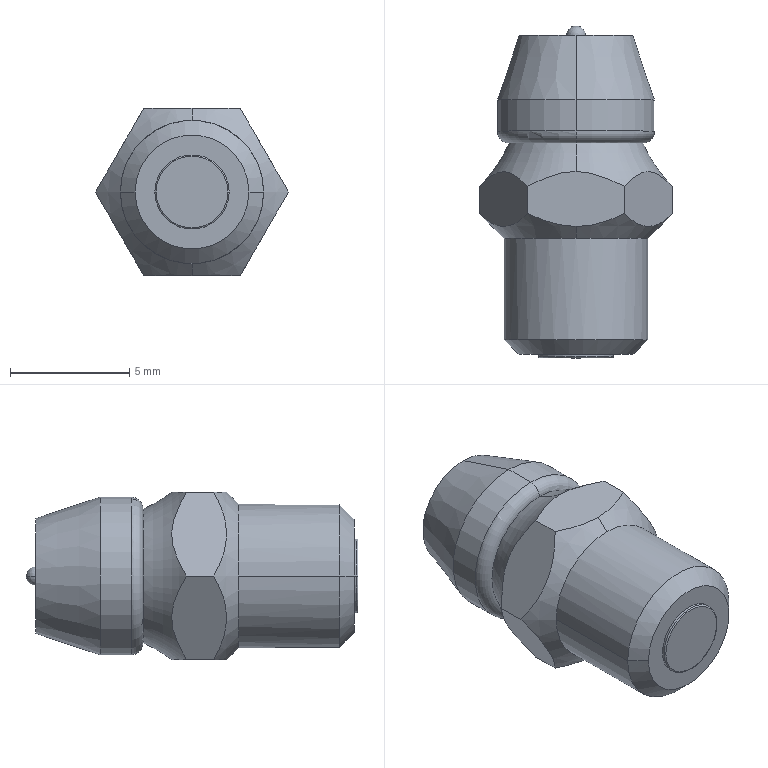Part | STEP file | GPAS6A-4 | 1 solid | 29 faces | box 8.083 x 13.9 x 7 mm | volume 414.719 mm3 | plane 9 | cylinder 6 | cone 6 | torus 6 | sphere 2 | commonest cylinder face diameters 3.113 x2 6 x2 6.6 x2
STEP:
#1=CARTESIAN_POINT('',(-3.,-5.986,0.));
#2=VERTEX_POINT('',#1);
#3=CARTESIAN_POINT('',(3.,-5.986,0.));
#4=VERTEX_POINT('',#3);
#5=CARTESIAN_POINT('',(0.,-5.986,0.));
#6=DIRECTION('',(0.,1.,0.));
#7=DIRECTION('',(-1.,0.,0.));
#8=AXIS2_PLACEMENT_3D('',#5,#6,#7);
#9=CIRCLE('',#8,3.);
#10=EDGE_CURVE('',#2,#4,#9,.T.);
#11=ORIENTED_EDGE('',*,*,#10,.T.);
#12=CARTESIAN_POINT('',(3.,-1.75,0.));
#13=VERTEX_POINT('',#12);
#14=CARTESIAN_POINT('',(3.,-1.75,0.));
#15=DIRECTION('',(0.,1.,0.));
#16=VECTOR('',#15,1000.);
#17=LINE('',#14,#16);
#18=EDGE_CURVE('',#4,#13,#17,.T.);
#19=ORIENTED_EDGE('',*,*,#18,.T.);
#20=CARTESIAN_POINT('',(0.,-1.75,3.));
#21=VERTEX_POINT('',#20);
#22=CARTESIAN_POINT('',(0.,-1.75,0.));
#23=DIRECTION('',(0.,1.,0.));
#24=DIRECTION('',(-1.,0.,0.));
#25=AXIS2_PLACEMENT_3D('',#22,#23,#24);
#26=CIRCLE('',#25,3.);
#27=EDGE_CURVE('',#21,#13,#26,.T.);
#28=ORIENTED_EDGE('',*,*,#27,.F.);
#29=CARTESIAN_POINT('',(-3.,-1.75,0.));
#30=VERTEX_POINT('',#29);
#31=CARTESIAN_POINT('',(0.,-1.75,0.));
#32=DIRECTION('',(0.,1.,0.));
#33=DIRECTION('',(-1.,0.,0.));
#34=AXIS2_PLACEMENT_3D('',#31,#32,#33);
#35=CIRCLE('',#34,3.);
#36=EDGE_CURVE('',#30,#21,#35,.T.);
#37=ORIENTED_EDGE('',*,*,#36,.F.);
#38=CARTESIAN_POINT('',(-3.,-1.75,0.));
#39=DIRECTION('',(0.,1.,0.));
#40=VECTOR('',#39,1000.);
#41=LINE('',#38,#40);
#42=EDGE_CURVE('',#2,#30,#41,.T.);
#43=ORIENTED_EDGE('',*,*,#42,.F.);
#44=EDGE_LOOP('',(#11,#19,#28,#37,#43));
#45=FACE_OUTER_BOUND('',#44,.T.);
#46=CARTESIAN_POINT('',(0.,-1.75,0.));
#47=DIRECTION('',(0.,1.,0.));
#48=DIRECTION('',(-1.,0.,0.));
#49=AXIS2_PLACEMENT_3D('',#46,#47,#48);
#50=CYLINDRICAL_SURFACE('',#49,3.);
#51=ADVANCED_FACE('',(#45),#50,.T.);
#52=CARTESIAN_POINT('',(-2.387,-6.6,0.));
#53=VERTEX_POINT('',#52);
#54=CARTESIAN_POINT('',(2.387,-6.6,0.));
#55=VERTEX_POINT('',#54);
#56=CARTESIAN_POINT('',(0.,-6.6,0.));
#57=DIRECTION('',(0.,1.,0.));
#58=DIRECTION('',(-1.,0.,0.));
#59=AXIS2_PLACEMENT_3D('',#56,#57,#58);
#60=CIRCLE('',#59,2.387);
#61=EDGE_CURVE('',#53,#55,#60,.T.);
#62=ORIENTED_EDGE('',*,*,#61,.T.);
#63=CARTESIAN_POINT('',(2.387,-6.6,0.));
#64=DIRECTION('',(0.7071,0.7071,0.));
#65=VECTOR('',#64,1000.);
#66=LINE('',#63,#65);
#67=EDGE_CURVE('',#55,#4,#66,.T.);
#68=ORIENTED_EDGE('',*,*,#67,.T.);
#69=ORIENTED_EDGE('',*,*,#10,.F.);
#70=CARTESIAN_POINT('',(-2.387,-6.6,0.));
#71=DIRECTION('',(-0.7071,0.7071,0.));
#72=VECTOR('',#71,1000.);
#73=LINE('',#70,#72);
#74=EDGE_CURVE('',#53,#2,#73,.T.);
#75=ORIENTED_EDGE('',*,*,#74,.F.);
#76=EDGE_LOOP('',(#62,#68,#69,#75));
#77=FACE_OUTER_BOUND('',#76,.T.);
#78=CARTESIAN_POINT('',(0.,-6.6,0.));
#79=DIRECTION('',(0.,1.,0.));
#80=DIRECTION('',(-1.,0.,0.));
#81=AXIS2_PLACEMENT_3D('',#78,#79,#80);
#82=CONICAL_SURFACE('',#81,2.387,0.7854);
#83=ADVANCED_FACE('',(#77),#82,.T.);
#84=CARTESIAN_POINT('',(-1.556,-6.698,0.));
#85=VERTEX_POINT('',#84);
#86=CARTESIAN_POINT('',(1.556,-6.698,0.));
#87=VERTEX_POINT('',#86);
#88=CARTESIAN_POINT('',(0.,-6.698,0.));
#89=DIRECTION('',(0.,1.,0.));
#90=DIRECTION('',(-1.,0.,0.));
#91=AXIS2_PLACEMENT_3D('',#88,#89,#90);
#92=CIRCLE('',#91,1.556);
#93=EDGE_CURVE('',#85,#87,#92,.T.);
#94=ORIENTED_EDGE('',*,*,#93,.T.);
#95=CARTESIAN_POINT('',(1.556,-6.6,0.));
#96=VERTEX_POINT('',#95);
#97=CARTESIAN_POINT('',(1.556,-1.75,0.));
#98=DIRECTION('',(0.,1.,0.));
#99=VECTOR('',#98,1000.);
#100=LINE('',#97,#99);
#101=EDGE_CURVE('',#87,#96,#100,.T.);
#102=ORIENTED_EDGE('',*,*,#101,.T.);
#103=CARTESIAN_POINT('',(-1.556,-6.6,0.));
#104=VERTEX_POINT('',#103);
#105=CARTESIAN_POINT('',(0.,-6.6,0.));
#106=DIRECTION('',(0.,1.,0.));
#107=DIRECTION('',(-1.,0.,0.));
#108=AXIS2_PLACEMENT_3D('',#105,#106,#107);
#109=CIRCLE('',#108,1.556);
#110=EDGE_CURVE('',#104,#96,#109,.T.);
#111=ORIENTED_EDGE('',*,*,#110,.F.);
#112=CARTESIAN_POINT('',(-1.556,-1.75,0.));
#113=DIRECTION('',(0.,1.,0.));
#114=VECTOR('',#113,1000.);
#115=LINE('',#112,#114);
#116=EDGE_CURVE('',#85,#104,#115,.T.);
#117=ORIENTED_EDGE('',*,*,#116,.F.);
#118=EDGE_LOOP('',(#94,#102,#111,#117));
#119=FACE_OUTER_BOUND('',#118,.T.);
#120=CARTESIAN_POINT('',(0.,-1.75,0.));
#121=DIRECTION('',(0.,1.,0.));
#122=DIRECTION('',(-1.,0.,0.));
#123=AXIS2_PLACEMENT_3D('',#120,#121,#122);
#124=CYLINDRICAL_SURFACE('',#123,1.556);
#125=ADVANCED_FACE('',(#119),#124,.T.);
#126=CARTESIAN_POINT('',(-1.505,-6.75,0.));
#127=VERTEX_POINT('',#126);
#128=CARTESIAN_POINT('',(1.505,-6.75,0.));
#129=VERTEX_POINT('',#128);
#130=CARTESIAN_POINT('',(0.,-6.75,0.));
#131=DIRECTION('',(0.,1.,0.));
#132=DIRECTION('',(-1.,0.,0.));
#133=AXIS2_PLACEMENT_3D('',#130,#131,#132);
#134=CIRCLE('',#133,1.505);
#135=EDGE_CURVE('',#127,#129,#134,.T.);
#136=ORIENTED_EDGE('',*,*,#135,.T.);
#137=CARTESIAN_POINT('',(1.505,-6.698,0.));
#138=DIRECTION('',(0.,0.,1.));
#139=DIRECTION('',(1.,0.,0.));
#140=AXIS2_PLACEMENT_3D('',#137,#138,#139);
#141=CIRCLE('',#140,0.05188);
#142=EDGE_CURVE('',#129,#87,#141,.T.);
#143=ORIENTED_EDGE('',*,*,#142,.T.);
#144=ORIENTED_EDGE('',*,*,#93,.F.);
#145=CARTESIAN_POINT('',(-1.505,-6.698,0.));
#146=DIRECTION('',(0.,0.,-1.));
#147=DIRECTION('',(-1.,0.,0.));
#148=AXIS2_PLACEMENT_3D('',#145,#146,#147);
#149=CIRCLE('',#148,0.05188);
#150=EDGE_CURVE('',#127,#85,#149,.T.);
#151=ORIENTED_EDGE('',*,*,#150,.F.);
#152=EDGE_LOOP('',(#136,#143,#144,#151));
#153=FACE_OUTER_BOUND('',#152,.T.);
#154=CARTESIAN_POINT('',(0.,-6.698,0.));
#155=DIRECTION('',(0.,1.,0.));
#156=DIRECTION('',(-1.,0.,0.));
#157=AXIS2_PLACEMENT_3D('',#154,#155,#156);
#158=TOROIDAL_SURFACE('',#157,1.505,0.05188);
#159=ADVANCED_FACE('',(#153),#158,.T.);
#160=CARTESIAN_POINT('',(0.4,6.75,0.));
#161=VERTEX_POINT('',#160);
#162=CARTESIAN_POINT('',(-0.4,6.75,0.));
#163=VERTEX_POINT('',#162);
#164=CARTESIAN_POINT('',(0.,6.75,0.));
#165=DIRECTION('',(0.,1.,0.));
#166=DIRECTION('',(0.,0.,1.));
#167=AXIS2_PLACEMENT_3D('',#164,#165,#166);
#168=CIRCLE('',#167,0.4);
#169=EDGE_CURVE('',#161,#163,#168,.T.);
#170=ORIENTED_EDGE('',*,*,#169,.T.);
#171=CARTESIAN_POINT('',(0.,7.15,0.));
#172=VERTEX_POINT('',#171);
#173=CARTESIAN_POINT('',(0.,6.75,0.));
#174=DIRECTION('',(0.,0.,-1.));
#175=DIRECTION('',(-1.,0.,0.));
#176=AXIS2_PLACEMENT_3D('',#173,#174,#175);
#177=CIRCLE('',#176,0.4);
#178=EDGE_CURVE('',#163,#172,#177,.T.);
#179=ORIENTED_EDGE('',*,*,#178,.T.);
#180=CARTESIAN_POINT('',(0.,6.75,0.));
#181=DIRECTION('',(0.,0.,1.));
#182=DIRECTION('',(1.,0.,0.));
#183=AXIS2_PLACEMENT_3D('',#180,#181,#182);
#184=CIRCLE('',#183,0.4);
#185=EDGE_CURVE('',#161,#172,#184,.T.);
#186=ORIENTED_EDGE('',*,*,#185,.F.);
#187=EDGE_LOOP('',(#170,#179,#186));
#188=FACE_OUTER_BOUND('',#187,.T.);
#189=CARTESIAN_POINT('',(0.,6.75,0.));
#190=DIRECTION('',(0.,0.,-1.));
#191=DIRECTION('',(1.,0.,0.));
#192=AXIS2_PLACEMENT_3D('',#189,#190,#191);
#193=SPHERICAL_SURFACE('',#192,0.4);
#194=ADVANCED_FACE('',(#188),#193,.T.);
#195=CARTESIAN_POINT('',(0.,6.75,2.4));
#196=VERTEX_POINT('',#195);
#197=CARTESIAN_POINT('',(0.,6.75,-2.4));
#198=VERTEX_POINT('',#197);
#199=CARTESIAN_POINT('',(0.,6.75,0.));
#200=DIRECTION('',(0.,1.,0.));
#201=DIRECTION('',(0.,0.,1.));
#202=AXIS2_PLACEMENT_3D('',#199,#200,#201);
#203=CIRCLE('',#202,2.4);
#204=EDGE_CURVE('',#196,#198,#203,.T.);
#205=ORIENTED_EDGE('',*,*,#204,.F.);
#206=CARTESIAN_POINT('',(0.,4.05,3.3));
#207=VERTEX_POINT('',#206);
#208=CARTESIAN_POINT('',(0.,4.05,3.3));
#209=DIRECTION('',(0.,-0.9487,0.3162));
#210=VECTOR('',#209,1000.);
#211=LINE('',#208,#210);
#212=EDGE_CURVE('',#196,#207,#211,.T.);
#213=ORIENTED_EDGE('',*,*,#212,.T.);
#214=CARTESIAN_POINT('',(0.,4.05,-3.3));
#215=VERTEX_POINT('',#214);
#216=CARTESIAN_POINT('',(0.,4.05,0.));
#217=DIRECTION('',(0.,1.,0.));
#218=DIRECTION('',(0.,0.,1.));
#219=AXIS2_PLACEMENT_3D('',#216,#217,#218);
#220=CIRCLE('',#219,3.3);
#221=EDGE_CURVE('',#207,#215,#220,.T.);
#222=ORIENTED_EDGE('',*,*,#221,.T.);
#223=CARTESIAN_POINT('',(0.,4.05,-3.3));
#224=DIRECTION('',(0.,-0.9487,-0.3162));
#225=VECTOR('',#224,1000.);
#226=LINE('',#223,#225);
#227=EDGE_CURVE('',#198,#215,#226,.T.);
#228=ORIENTED_EDGE('',*,*,#227,.F.);
#229=EDGE_LOOP('',(#205,#213,#222,#228));
#230=FACE_OUTER_BOUND('',#229,.T.);
#231=CARTESIAN_POINT('',(0.,4.05,0.));
#232=DIRECTION('',(0.,-1.,0.));
#233=DIRECTION('',(0.,0.,-1.));
#234=AXIS2_PLACEMENT_3D('',#231,#232,#233);
#235=CONICAL_SURFACE('',#234,3.3,0.3218);
#236=ADVANCED_FACE('',(#230),#235,.T.);
#237=CARTESIAN_POINT('',(0.,2.75,3.3));
#238=VERTEX_POINT('',#237);
#239=CARTESIAN_POINT('',(0.,2.75,-3.3));
#240=VERTEX_POINT('',#239);
#241=CARTESIAN_POINT('',(0.,2.75,0.));
#242=DIRECTION('',(0.,1.,0.));
#243=DIRECTION('',(0.,0.,1.));
#244=AXIS2_PLACEMENT_3D('',#241,#242,#243);
#245=CIRCLE('',#244,3.3);
#246=EDGE_CURVE('',#238,#240,#245,.T.);
#247=ORIENTED_EDGE('',*,*,#246,.T.);
#248=CARTESIAN_POINT('',(0.,6.75,-3.3));
#249=DIRECTION('',(0.,1.,0.));
#250=VECTOR('',#249,1000.);
#251=LINE('',#248,#250);
#252=EDGE_CURVE('',#240,#215,#251,.T.);
#253=ORIENTED_EDGE('',*,*,#252,.T.);
#254=ORIENTED_EDGE('',*,*,#221,.F.);
#255=CARTESIAN_POINT('',(0.,6.75,3.3));
#256=DIRECTION('',(0.,1.,0.));
#257=VECTOR('',#256,1000.);
#258=LINE('',#255,#257);
#259=EDGE_CURVE('',#238,#207,#258,.T.);
#260=ORIENTED_EDGE('',*,*,#259,.F.);
#261=EDGE_LOOP('',(#247,#253,#254,#260));
#262=FACE_OUTER_BOUND('',#261,.T.);
#263=CARTESIAN_POINT('',(0.,6.75,0.));
#264=DIRECTION('',(0.,1.,0.));
#265=DIRECTION('',(0.,0.,1.));
#266=AXIS2_PLACEMENT_3D('',#263,#264,#265);
#267=CYLINDRICAL_SURFACE('',#266,3.3);
#268=ADVANCED_FACE('',(#262),#267,.T.);
#269=CARTESIAN_POINT('',(0.,2.25,2.8));
#270=VERTEX_POINT('',#269);
#271=CARTESIAN_POINT('',(0.,2.25,-2.8));
#272=VERTEX_POINT('',#271);
#273=CARTESIAN_POINT('',(0.,2.25,0.));
#274=DIRECTION('',(0.,1.,0.));
#275=DIRECTION('',(0.,0.,1.));
#276=AXIS2_PLACEMENT_3D('',#273,#274,#275);
#277=CIRCLE('',#276,2.8);
#278=EDGE_CURVE('',#270,#272,#277,.T.);
#279=ORIENTED_EDGE('',*,*,#278,.T.);
#280=CARTESIAN_POINT('',(0.,2.75,-2.8));
#281=DIRECTION('',(1.,0.,0.));
#282=DIRECTION('',(0.,0.,-1.));
#283=AXIS2_PLACEMENT_3D('',#280,#281,#282);
#284=CIRCLE('',#283,0.5);
#285=EDGE_CURVE('',#272,#240,#284,.T.);
#286=ORIENTED_EDGE('',*,*,#285,.T.);
#287=ORIENTED_EDGE('',*,*,#246,.F.);
#288=CARTESIAN_POINT('',(0.,2.75,2.8));
#289=DIRECTION('',(-1.,0.,0.));
#290=DIRECTION('',(0.,0.,1.));
#291=AXIS2_PLACEMENT_3D('',#288,#289,#290);
#292=CIRCLE('',#291,0.5);
#293=EDGE_CURVE('',#270,#238,#292,.T.);
#294=ORIENTED_EDGE('',*,*,#293,.F.);
#295=EDGE_LOOP('',(#279,#286,#287,#294));
#296=FACE_OUTER_BOUND('',#295,.T.);
#297=CARTESIAN_POINT('',(0.,2.75,0.));
#298=DIRECTION('',(0.,1.,0.));
#299=DIRECTION('',(0.,0.,1.));
#300=AXIS2_PLACEMENT_3D('',#297,#298,#299);
#301=TOROIDAL_SURFACE('',#300,2.8,0.5);
#302=ADVANCED_FACE('',(#296),#301,.T.);
#303=CARTESIAN_POINT('',(0.,2.25,0.));
#304=DIRECTION('',(0.,1.,0.));
#305=DIRECTION('',(0.,0.,1.));
#306=AXIS2_PLACEMENT_3D('',#303,#304,#305);
#307=CIRCLE('',#306,2.8);
#308=EDGE_CURVE('',#272,#270,#307,.T.);
#309=ORIENTED_EDGE('',*,*,#308,.F.);
#310=CARTESIAN_POINT('',(0.,1.053,-3.5));
#311=VERTEX_POINT('',#310);
#312=CARTESIAN_POINT('',(0.,4.661,-8.294));
#313=DIRECTION('',(1.,0.,0.));
#314=DIRECTION('',(0.,0.,-1.));
#315=AXIS2_PLACEMENT_3D('',#312,#313,#314);
#316=CIRCLE('',#315,6.);
#317=EDGE_CURVE('',#272,#311,#316,.T.);
#318=ORIENTED_EDGE('',*,*,#317,.T.);
#319=CARTESIAN_POINT('',(-2.021,0.4286,-3.5));
#320=VERTEX_POINT('',#319);
#321=CARTESIAN_POINT('',(0.,1.053,-3.5));
#322=CARTESIAN_POINT('',(-0.1777,1.053,-3.5));
#323=CARTESIAN_POINT('',(-0.3562,1.035,-3.5));
#324=CARTESIAN_POINT('',(-0.7092,0.9659,-3.5));
#325=CARTESIAN_POINT('',(-0.88,0.9167,-3.5));
#326=CARTESIAN_POINT('',(-1.382,0.7411,-3.5));
#327=CARTESIAN_POINT('',(-1.703,0.5884,-3.5));
#328=CARTESIAN_POINT('',(-2.021,0.4286,-3.5));
#329=B_SPLINE_CURVE_WITH_KNOTS('',3,(#321,#322,#323,#324,#325,#326,#327,#328),.UNSPECIFIED.,.F.,.F.,(4,2,2,4),(0.00693,0.007463,0.007996,0.009062),.UNSPECIFIED.);
#330=EDGE_CURVE('',#311,#320,#329,.T.);
#331=ORIENTED_EDGE('',*,*,#330,.T.);
#332=CARTESIAN_POINT('',(-4.041,0.4286,0.));
#333=VERTEX_POINT('',#332);
#334=CARTESIAN_POINT('',(-2.021,0.4286,-3.5));
#335=CARTESIAN_POINT('',(-2.18,0.5886,-3.224));
#336=CARTESIAN_POINT('',(-2.341,0.7417,-2.946));
#337=CARTESIAN_POINT('',(-2.593,0.9177,-2.509));
#338=CARTESIAN_POINT('',(-2.679,0.9672,-2.359));
#339=CARTESIAN_POINT('',(-2.854,1.035,-2.057));
#340=CARTESIAN_POINT('',(-2.942,1.053,-1.904));
#341=CARTESIAN_POINT('',(-3.12,1.053,-1.597));
#342=CARTESIAN_POINT('',(-3.21,1.035,-1.441));
#343=CARTESIAN_POINT('',(-3.384,0.9667,-1.139));
#344=CARTESIAN_POINT('',(-3.469,0.9179,-0.9914));
#345=CARTESIAN_POINT('',(-3.72,0.7428,-0.5566));
#346=CARTESIAN_POINT('',(-3.882,0.5887,-0.2761));
#347=CARTESIAN_POINT('',(-4.041,0.4286,0.));
#348=B_SPLINE_CURVE_WITH_KNOTS('',3,(#334,#335,#336,#337,#338,#339,#340,#341,#342,#343,#344,#345,#346,#347),.UNSPECIFIED.,.F.,.F.,(4,2,2,2,2,2,4),(0.000000258,0.001066,0.001599,0.002132,0.002666,0.003199,0.004265),.UNSPECIFIED.);
#349=EDGE_CURVE('',#320,#333,#348,.T.);
#350=ORIENTED_EDGE('',*,*,#349,.T.);
#351=CARTESIAN_POINT('',(-2.021,0.4286,3.5));
#352=VERTEX_POINT('',#351);
#353=CARTESIAN_POINT('',(-4.041,0.4286,0.));
#354=CARTESIAN_POINT('',(-3.882,0.5886,0.2759));
#355=CARTESIAN_POINT('',(-3.721,0.7417,0.5542));
#356=CARTESIAN_POINT('',(-3.47,0.9177,0.9906));
#357=CARTESIAN_POINT('',(-3.383,0.9672,1.141));
#358=CARTESIAN_POINT('',(-3.208,1.035,1.443));
#359=CARTESIAN_POINT('',(-3.12,1.053,1.596));
#360=CARTESIAN_POINT('',(-2.943,1.053,1.903));
#361=CARTESIAN_POINT('',(-2.853,1.035,2.059));
#362=CARTESIAN_POINT('',(-2.678,0.9667,2.361));
#363=CARTESIAN_POINT('',(-2.593,0.9179,2.509));
#364=CARTESIAN_POINT('',(-2.342,0.7428,2.943));
#365=CARTESIAN_POINT('',(-2.18,0.5887,3.224));
#366=CARTESIAN_POINT('',(-2.021,0.4286,3.5));
#367=B_SPLINE_CURVE_WITH_KNOTS('',3,(#353,#354,#355,#356,#357,#358,#359,#360,#361,#362,#363,#364,#365,#366),.UNSPECIFIED.,.F.,.F.,(4,2,2,2,2,2,4),(0.000000258,0.001066,0.001599,0.002132,0.002666,0.003199,0.004265),.UNSPECIFIED.);
#368=EDGE_CURVE('',#333,#352,#367,.T.);
#369=ORIENTED_EDGE('',*,*,#368,.T.);
#370=CARTESIAN_POINT('',(0.,1.053,3.5));
#371=VERTEX_POINT('',#370);
#372=CARTESIAN_POINT('',(-2.021,0.4286,3.5));
#373=CARTESIAN_POINT('',(-1.702,0.5886,3.5));
#374=CARTESIAN_POINT('',(-1.379,0.7424,3.5));
#375=CARTESIAN_POINT('',(-0.8765,0.9178,3.5));
#376=CARTESIAN_POINT('',(-0.7058,0.9668,3.5));
#377=CARTESIAN_POINT('',(-0.3544,1.035,3.5));
#378=CARTESIAN_POINT('',(-0.1767,1.053,3.5));
#379=CARTESIAN_POINT('',(0.,1.053,3.5));
#380=B_SPLINE_CURVE_WITH_KNOTS('',3,(#372,#373,#374,#375,#376,#377,#378,#379),.UNSPECIFIED.,.F.,.F.,(4,2,2,4),(0.004809,0.00587,0.0064,0.00693),.UNSPECIFIED.);
#381=EDGE_CURVE('',#352,#371,#380,.T.);
#382=ORIENTED_EDGE('',*,*,#381,.T.);
#383=CARTESIAN_POINT('',(0.,4.661,8.294));
#384=DIRECTION('',(-1.,0.,0.));
#385=DIRECTION('',(0.,0.,1.));
#386=AXIS2_PLACEMENT_3D('',#383,#384,#385);
#387=CIRCLE('',#386,6.);
#388=EDGE_CURVE('',#270,#371,#387,.T.);
#389=ORIENTED_EDGE('',*,*,#388,.F.);
#390=EDGE_LOOP('',(#309,#318,#331,#350,#369,#382,#389));
#391=FACE_OUTER_BOUND('',#390,.T.);
#392=CARTESIAN_POINT('',(0.,4.661,0.));
#393=DIRECTION('',(0.,1.,0.));
#394=DIRECTION('',(0.,0.,1.));
#395=AXIS2_PLACEMENT_3D('',#392,#393,#394);
#396=TOROIDAL_SURFACE('',#395,8.294,6.);
#397=ADVANCED_FACE('',(#391),#396,.F.);
#398=ORIENTED_EDGE('',*,*,#27,.T.);
#399=CARTESIAN_POINT('',(0.,-1.75,-3.));
#400=VERTEX_POINT('',#399);
#401=CARTESIAN_POINT('',(0.,-1.75,0.));
#402=DIRECTION('',(0.,1.,0.));
#403=DIRECTION('',(-1.,0.,0.));
#404=AXIS2_PLACEMENT_3D('',#401,#402,#403);
#405=CIRCLE('',#404,3.);
#406=EDGE_CURVE('',#13,#400,#405,.T.);
#407=ORIENTED_EDGE('',*,*,#406,.T.);
#408=CARTESIAN_POINT('',(0.,-1.25,-3.5));
#409=VERTEX_POINT('',#408);
#410=CARTESIAN_POINT('',(0.,-1.8,-2.95));
#411=DIRECTION('',(0.,0.7071,-0.7071));
#412=VECTOR('',#411,1000.);
#413=LINE('',#410,#412);
#414=EDGE_CURVE('',#400,#409,#413,.T.);
#415=ORIENTED_EDGE('',*,*,#414,.T.);
#416=CARTESIAN_POINT('',(2.021,-0.7085,-3.5));
#417=VERTEX_POINT('',#416);
#418=CARTESIAN_POINT('',(0.,-1.25,-3.5));
#419=CARTESIAN_POINT('',(0.1774,-1.25,-3.5));
#420=CARTESIAN_POINT('',(0.3548,-1.236,-3.5));
#421=CARTESIAN_POINT('',(0.7015,-1.185,-3.5));
#422=CARTESIAN_POINT('',(0.8722,-1.147,-3.5));
#423=CARTESIAN_POINT('',(1.377,-1.003,-3.5));
#424=CARTESIAN_POINT('',(1.707,-0.8653,-3.5));
#425=CARTESIAN_POINT('',(2.021,-0.7085,-3.5));
#426=B_SPLINE_CURVE_WITH_KNOTS('',3,(#418,#419,#420,#421,#422,#423,#424,#425),.UNSPECIFIED.,.F.,.F.,(4,2,2,4),(0.007385,0.007911,0.008437,0.009489),.UNSPECIFIED.);
#427=EDGE_CURVE('',#409,#417,#426,.T.);
#428=ORIENTED_EDGE('',*,*,#427,.T.);
#429=CARTESIAN_POINT('',(4.041,-0.7085,0.));
#430=VERTEX_POINT('',#429);
#431=CARTESIAN_POINT('',(2.021,-0.7085,-3.5));
#432=CARTESIAN_POINT('',(2.179,-0.8664,-3.227));
#433=CARTESIAN_POINT('',(2.34,-1.001,-2.947));
#434=CARTESIAN_POINT('',(2.591,-1.145,-2.512));
#435=CARTESIAN_POINT('',(2.676,-1.183,-2.365));
#436=CARTESIAN_POINT('',(2.85,-1.235,-2.064));
#437=CARTESIAN_POINT('',(2.939,-1.25,-1.909));
#438=CARTESIAN_POINT('',(3.204,-1.251,-1.451));
#439=CARTESIAN_POINT('',(3.377,-1.197,-1.151));
#440=CARTESIAN_POINT('',(3.719,-1.004,-0.5583));
#441=CARTESIAN_POINT('',(3.883,-0.8674,-0.2751));
#442=CARTESIAN_POINT('',(4.041,-0.7085,0.));
#443=B_SPLINE_CURVE_WITH_KNOTS('',3,(#431,#432,#433,#434,#435,#436,#437,#438,#439,#440,#441,#442),.UNSPECIFIED.,.F.,.F.,(4,2,2,2,2,4),(0.000000254,0.001044,0.001566,0.002088,0.003131,0.004175),.UNSPECIFIED.);
#444=EDGE_CURVE('',#417,#430,#443,.T.);
#445=ORIENTED_EDGE('',*,*,#444,.T.);
#446=CARTESIAN_POINT('',(2.021,-0.7085,3.5));
#447=VERTEX_POINT('',#446);
#448=CARTESIAN_POINT('',(4.041,-0.7085,0.));
#449=CARTESIAN_POINT('',(3.884,-0.8664,0.2735));
#450=CARTESIAN_POINT('',(3.722,-1.001,0.5531));
#451=CARTESIAN_POINT('',(3.471,-1.145,0.9875));
#452=CARTESIAN_POINT('',(3.386,-1.183,1.135));
#453=CARTESIAN_POINT('',(3.212,-1.235,1.436));
#454=CARTESIAN_POINT('',(3.123,-1.25,1.591));
#455=CARTESIAN_POINT('',(2.858,-1.251,2.049));
#456=CARTESIAN_POINT('',(2.685,-1.197,2.349));
#457=CARTESIAN_POINT('',(2.343,-1.004,2.942));
#458=CARTESIAN_POINT('',(2.18,-0.8674,3.225));
#459=CARTESIAN_POINT('',(2.021,-0.7085,3.5));
#460=B_SPLINE_CURVE_WITH_KNOTS('',3,(#448,#449,#450,#451,#452,#453,#454,#455,#456,#457,#458,#459),.UNSPECIFIED.,.F.,.F.,(4,2,2,2,2,4),(0.000000254,0.001044,0.001566,0.002088,0.003131,0.004175),.UNSPECIFIED.);
#461=EDGE_CURVE('',#430,#447,#460,.T.);
#462=ORIENTED_EDGE('',*,*,#461,.T.);
#463=CARTESIAN_POINT('',(0.,-1.25,3.5));
#464=VERTEX_POINT('',#463);
#465=CARTESIAN_POINT('',(2.021,-0.7085,3.5));
#466=CARTESIAN_POINT('',(1.864,-0.7869,3.5));
#467=CARTESIAN_POINT('',(1.704,-0.8601,3.5));
#468=CARTESIAN_POINT('',(1.376,-0.9922,3.5));
#469=CARTESIAN_POINT('',(1.208,-1.051,3.5));
#470=CARTESIAN_POINT('',(0.7009,-1.195,3.5));
#471=CARTESIAN_POINT('',(0.3554,-1.25,3.5));
#472=CARTESIAN_POINT('',(0.,-1.25,3.5));
#473=B_SPLINE_CURVE_WITH_KNOTS('',3,(#465,#466,#467,#468,#469,#470,#471,#472),.UNSPECIFIED.,.F.,.F.,(4,2,2,4),(0.005277,0.005804,0.006331,0.007385),.UNSPECIFIED.);
#474=EDGE_CURVE('',#447,#464,#473,.T.);
#475=ORIENTED_EDGE('',*,*,#474,.T.);
#476=CARTESIAN_POINT('',(0.,-1.8,2.95));
#477=DIRECTION('',(0.,0.7071,0.7071));
#478=VECTOR('',#477,1000.);
#479=LINE('',#476,#478);
#480=EDGE_CURVE('',#21,#464,#479,.T.);
#481=ORIENTED_EDGE('',*,*,#480,.F.);
#482=EDGE_LOOP('',(#398,#407,#415,#428,#445,#462,#475,#481));
#483=FACE_OUTER_BOUND('',#482,.T.);
#484=CARTESIAN_POINT('',(0.,-1.8,0.));
#485=DIRECTION('',(0.,1.,0.));
#486=DIRECTION('',(0.,0.,1.));
#487=AXIS2_PLACEMENT_3D('',#484,#485,#486);
#488=CONICAL_SURFACE('',#487,2.95,0.7854);
#489=ADVANCED_FACE('',(#483),#488,.T.);
#490=ORIENTED_EDGE('',*,*,#414,.F.);
#491=CARTESIAN_POINT('',(0.,-1.75,0.));
#492=DIRECTION('',(0.,1.,0.));
#493=DIRECTION('',(-1.,0.,0.));
#494=AXIS2_PLACEMENT_3D('',#491,#492,#493);
#495=CIRCLE('',#494,3.);
#496=EDGE_CURVE('',#400,#30,#495,.T.);
#497=ORIENTED_EDGE('',*,*,#496,.T.);
#498=ORIENTED_EDGE('',*,*,#36,.T.);
#499=ORIENTED_EDGE('',*,*,#480,.T.);
#500=CARTESIAN_POINT('',(-2.021,-0.7085,3.5));
#501=VERTEX_POINT('',#500);
#502=CARTESIAN_POINT('',(0.,-1.25,3.5));
#503=CARTESIAN_POINT('',(-0.1774,-1.25,3.5));
#504=CARTESIAN_POINT('',(-0.3548,-1.236,3.5));
#505=CARTESIAN_POINT('',(-0.7015,-1.185,3.5));
#506=CARTESIAN_POINT('',(-0.8722,-1.147,3.5));
#507=CARTESIAN_POINT('',(-1.377,-1.003,3.5));
#508=CARTESIAN_POINT('',(-1.707,-0.8653,3.5));
#509=CARTESIAN_POINT('',(-2.021,-0.7085,3.5));
#510=B_SPLINE_CURVE_WITH_KNOTS('',3,(#502,#503,#504,#505,#506,#507,#508,#509),.UNSPECIFIED.,.F.,.F.,(4,2,2,4),(0.007385,0.007911,0.008437,0.009489),.UNSPECIFIED.);
#511=EDGE_CURVE('',#464,#501,#510,.T.);
#512=ORIENTED_EDGE('',*,*,#511,.T.);
#513=CARTESIAN_POINT('',(-4.041,-0.7085,0.));
#514=VERTEX_POINT('',#513);
#515=CARTESIAN_POINT('',(-2.021,-0.7085,3.5));
#516=CARTESIAN_POINT('',(-2.179,-0.8664,3.227));
#517=CARTESIAN_POINT('',(-2.34,-1.001,2.947));
#518=CARTESIAN_POINT('',(-2.591,-1.145,2.512));
#519=CARTESIAN_POINT('',(-2.676,-1.183,2.365));
#520=CARTESIAN_POINT('',(-2.85,-1.235,2.064));
#521=CARTESIAN_POINT('',(-2.939,-1.25,1.909));
#522=CARTESIAN_POINT('',(-3.204,-1.251,1.451));
#523=CARTESIAN_POINT('',(-3.377,-1.197,1.151));
#524=CARTESIAN_POINT('',(-3.719,-1.004,0.5583));
#525=CARTESIAN_POINT('',(-3.883,-0.8674,0.2751));
#526=CARTESIAN_POINT('',(-4.041,-0.7085,0.));
#527=B_SPLINE_CURVE_WITH_KNOTS('',3,(#515,#516,#517,#518,#519,#520,#521,#522,#523,#524,#525,#526),.UNSPECIFIED.,.F.,.F.,(4,2,2,2,2,4),(0.000000254,0.001044,0.001566,0.002088,0.003131,0.004175),.UNSPECIFIED.);
#528=EDGE_CURVE('',#501,#514,#527,.T.);
#529=ORIENTED_EDGE('',*,*,#528,.T.);
#530=CARTESIAN_POINT('',(-2.021,-0.7085,-3.5));
#531=VERTEX_POINT('',#530);
#532=CARTESIAN_POINT('',(-4.041,-0.7085,0.));
#533=CARTESIAN_POINT('',(-3.884,-0.8664,-0.2735));
#534=CARTESIAN_POINT('',(-3.722,-1.001,-0.5531));
#535=CARTESIAN_POINT('',(-3.471,-1.145,-0.9875));
#536=CARTESIAN_POINT('',(-3.386,-1.183,-1.135));
#537=CARTESIAN_POINT('',(-3.212,-1.235,-1.436));
#538=CARTESIAN_POINT('',(-3.123,-1.25,-1.591));
#539=CARTESIAN_POINT('',(-2.858,-1.251,-2.049));
#540=CARTESIAN_POINT('',(-2.685,-1.197,-2.349));
#541=CARTESIAN_POINT('',(-2.343,-1.004,-2.942));
#542=CARTESIAN_POINT('',(-2.18,-0.8674,-3.225));
#543=CARTESIAN_POINT('',(-2.021,-0.7085,-3.5));
#544=B_SPLINE_CURVE_WITH_KNOTS('',3,(#532,#533,#534,#535,#536,#537,#538,#539,#540,#541,#542,#543),.UNSPECIFIED.,.F.,.F.,(4,2,2,2,2,4),(0.000000254,0.001044,0.001566,0.002088,0.003131,0.004175),.UNSPECIFIED.);
#545=EDGE_CURVE('',#514,#531,#544,.T.);
#546=ORIENTED_EDGE('',*,*,#545,.T.);
#547=CARTESIAN_POINT('',(-2.021,-0.7085,-3.5));
#548=CARTESIAN_POINT('',(-1.864,-0.7869,-3.5));
#549=CARTESIAN_POINT('',(-1.704,-0.8601,-3.5));
#550=CARTESIAN_POINT('',(-1.376,-0.9922,-3.5));
#551=CARTESIAN_POINT('',(-1.208,-1.051,-3.5));
#552=CARTESIAN_POINT('',(-0.7009,-1.195,-3.5));
#553=CARTESIAN_POINT('',(-0.3554,-1.25,-3.5));
#554=CARTESIAN_POINT('',(0.,-1.25,-3.5));
#555=B_SPLINE_CURVE_WITH_KNOTS('',3,(#547,#548,#549,#550,#551,#552,#553,#554),.UNSPECIFIED.,.F.,.F.,(4,2,2,4),(0.005277,0.005804,0.006331,0.007385),.UNSPECIFIED.);
#556=EDGE_CURVE('',#531,#409,#555,.T.);
#557=ORIENTED_EDGE('',*,*,#556,.T.);
#558=EDGE_LOOP('',(#490,#497,#498,#499,#512,#529,#546,#557));
#559=FACE_OUTER_BOUND('',#558,.T.);
#560=CARTESIAN_POINT('',(0.,-1.8,0.));
#561=DIRECTION('',(0.,1.,0.));
#562=DIRECTION('',(0.,0.,1.));
#563=AXIS2_PLACEMENT_3D('',#560,#561,#562);
#564=CONICAL_SURFACE('',#563,2.95,0.7854);
#565=ADVANCED_FACE('',(#559),#564,.T.);
#566=ORIENTED_EDGE('',*,*,#317,.F.);
#567=ORIENTED_EDGE('',*,*,#278,.F.);
#568=ORIENTED_EDGE('',*,*,#388,.T.);
#569=CARTESIAN_POINT('',(2.021,0.4286,3.5));
#570=VERTEX_POINT('',#569);
#571=CARTESIAN_POINT('',(0.,1.053,3.5));
#572=CARTESIAN_POINT('',(0.1777,1.053,3.5));
#573=CARTESIAN_POINT('',(0.3562,1.035,3.5));
#574=CARTESIAN_POINT('',(0.7092,0.9659,3.5));
#575=CARTESIAN_POINT('',(0.88,0.9167,3.5));
#576=CARTESIAN_POINT('',(1.382,0.7411,3.5));
#577=CARTESIAN_POINT('',(1.703,0.5884,3.5));
#578=CARTESIAN_POINT('',(2.021,0.4286,3.5));
#579=B_SPLINE_CURVE_WITH_KNOTS('',3,(#571,#572,#573,#574,#575,#576,#577,#578),.UNSPECIFIED.,.F.,.F.,(4,2,2,4),(0.00693,0.007463,0.007996,0.009062),.UNSPECIFIED.);
#580=EDGE_CURVE('',#371,#570,#579,.T.);
#581=ORIENTED_EDGE('',*,*,#580,.T.);
#582=CARTESIAN_POINT('',(4.041,0.4286,0.));
#583=VERTEX_POINT('',#582);
#584=CARTESIAN_POINT('',(2.021,0.4286,3.5));
#585=CARTESIAN_POINT('',(2.18,0.5886,3.224));
#586=CARTESIAN_POINT('',(2.341,0.7417,2.946));
#587=CARTESIAN_POINT('',(2.593,0.9177,2.509));
#588=CARTESIAN_POINT('',(2.679,0.9672,2.359));
#589=CARTESIAN_POINT('',(2.854,1.035,2.057));
#590=CARTESIAN_POINT('',(2.942,1.053,1.904));
#591=CARTESIAN_POINT('',(3.12,1.053,1.597));
#592=CARTESIAN_POINT('',(3.21,1.035,1.441));
#593=CARTESIAN_POINT('',(3.384,0.9667,1.139));
#594=CARTESIAN_POINT('',(3.469,0.9179,0.9914));
#595=CARTESIAN_POINT('',(3.72,0.7428,0.5566));
#596=CARTESIAN_POINT('',(3.882,0.5887,0.2761));
#597=CARTESIAN_POINT('',(4.041,0.4286,0.));
#598=B_SPLINE_CURVE_WITH_KNOTS('',3,(#584,#585,#586,#587,#588,#589,#590,#591,#592,#593,#594,#595,#596,#597),.UNSPECIFIED.,.F.,.F.,(4,2,2,2,2,2,4),(0.000000258,0.001066,0.001599,0.002132,0.002666,0.003199,0.004265),.UNSPECIFIED.);
#599=EDGE_CURVE('',#570,#583,#598,.T.);
#600=ORIENTED_EDGE('',*,*,#599,.T.);
#601=CARTESIAN_POINT('',(2.021,0.4286,-3.5));
#602=VERTEX_POINT('',#601);
#603=CARTESIAN_POINT('',(4.041,0.4286,0.));
#604=CARTESIAN_POINT('',(3.882,0.5886,-0.2759));
#605=CARTESIAN_POINT('',(3.721,0.7417,-0.5542));
#606=CARTESIAN_POINT('',(3.47,0.9177,-0.9906));
#607=CARTESIAN_POINT('',(3.383,0.9672,-1.141));
#608=CARTESIAN_POINT('',(3.208,1.035,-1.443));
#609=CARTESIAN_POINT('',(3.12,1.053,-1.596));
#610=CARTESIAN_POINT('',(2.943,1.053,-1.903));
#611=CARTESIAN_POINT('',(2.853,1.035,-2.059));
#612=CARTESIAN_POINT('',(2.678,0.9667,-2.361));
#613=CARTESIAN_POINT('',(2.593,0.9179,-2.509));
#614=CARTESIAN_POINT('',(2.342,0.7428,-2.943));
#615=CARTESIAN_POINT('',(2.18,0.5887,-3.224));
#616=CARTESIAN_POINT('',(2.021,0.4286,-3.5));
#617=B_SPLINE_CURVE_WITH_KNOTS('',3,(#603,#604,#605,#606,#607,#608,#609,#610,#611,#612,#613,#614,#615,#616),.UNSPECIFIED.,.F.,.F.,(4,2,2,2,2,2,4),(0.000000258,0.001066,0.001599,0.002132,0.002666,0.003199,0.004265),.UNSPECIFIED.);
#618=EDGE_CURVE('',#583,#602,#617,.T.);
#619=ORIENTED_EDGE('',*,*,#618,.T.);
#620=CARTESIAN_POINT('',(2.021,0.4286,-3.5));
#621=CARTESIAN_POINT('',(1.702,0.5886,-3.5));
#622=CARTESIAN_POINT('',(1.379,0.7424,-3.5));
#623=CARTESIAN_POINT('',(0.8765,0.9178,-3.5));
#624=CARTESIAN_POINT('',(0.7058,0.9668,-3.5));
#625=CARTESIAN_POINT('',(0.3544,1.035,-3.5));
#626=CARTESIAN_POINT('',(0.1767,1.053,-3.5));
#627=CARTESIAN_POINT('',(0.,1.053,-3.5));
#628=B_SPLINE_CURVE_WITH_KNOTS('',3,(#620,#621,#622,#623,#624,#625,#626,#627),.UNSPECIFIED.,.F.,.F.,(4,2,2,4),(0.004809,0.00587,0.0064,0.00693),.UNSPECIFIED.);
#629=EDGE_CURVE('',#602,#311,#628,.T.);
#630=ORIENTED_EDGE('',*,*,#629,.T.);
#631=EDGE_LOOP('',(#566,#567,#568,#581,#600,#619,#630));
#632=FACE_OUTER_BOUND('',#631,.T.);
#633=CARTESIAN_POINT('',(0.,4.661,0.));
#634=DIRECTION('',(0.,1.,0.));
#635=DIRECTION('',(0.,0.,1.));
#636=AXIS2_PLACEMENT_3D('',#633,#634,#635);
#637=TOROIDAL_SURFACE('',#636,8.294,6.);
#638=ADVANCED_FACE('',(#632),#637,.F.);
#639=ORIENTED_EDGE('',*,*,#285,.F.);
#640=ORIENTED_EDGE('',*,*,#308,.T.);
#641=ORIENTED_EDGE('',*,*,#293,.T.);
#642=CARTESIAN_POINT('',(0.,2.75,0.));
#643=DIRECTION('',(0.,1.,0.));
#644=DIRECTION('',(0.,0.,1.));
#645=AXIS2_PLACEMENT_3D('',#642,#643,#644);
#646=CIRCLE('',#645,3.3);
#647=EDGE_CURVE('',#240,#238,#646,.T.);
#648=ORIENTED_EDGE('',*,*,#647,.F.);
#649=EDGE_LOOP('',(#639,#640,#641,#648));
#650=FACE_OUTER_BOUND('',#649,.T.);
#651=CARTESIAN_POINT('',(0.,2.75,0.));
#652=DIRECTION('',(0.,1.,0.));
#653=DIRECTION('',(0.,0.,1.));
#654=AXIS2_PLACEMENT_3D('',#651,#652,#653);
#655=TOROIDAL_SURFACE('',#654,2.8,0.5);
#656=ADVANCED_FACE('',(#650),#655,.T.);
#657=ORIENTED_EDGE('',*,*,#252,.F.);
#658=ORIENTED_EDGE('',*,*,#647,.T.);
#659=ORIENTED_EDGE('',*,*,#259,.T.);
#660=CARTESIAN_POINT('',(0.,4.05,0.));
#661=DIRECTION('',(0.,1.,0.));
#662=DIRECTION('',(0.,0.,1.));
#663=AXIS2_PLACEMENT_3D('',#660,#661,#662);
#664=CIRCLE('',#663,3.3);
#665=EDGE_CURVE('',#215,#207,#664,.T.);
#666=ORIENTED_EDGE('',*,*,#665,.F.);
#667=EDGE_LOOP('',(#657,#658,#659,#666));
#668=FACE_OUTER_BOUND('',#667,.T.);
#669=CARTESIAN_POINT('',(0.,6.75,0.));
#670=DIRECTION('',(0.,1.,0.));
#671=DIRECTION('',(0.,0.,1.));
#672=AXIS2_PLACEMENT_3D('',#669,#670,#671);
#673=CYLINDRICAL_SURFACE('',#672,3.3);
#674=ADVANCED_FACE('',(#668),#673,.T.);
#675=ORIENTED_EDGE('',*,*,#212,.F.);
#676=CARTESIAN_POINT('',(0.,6.75,0.));
#677=DIRECTION('',(0.,1.,0.));
#678=DIRECTION('',(0.,0.,1.));
#679=AXIS2_PLACEMENT_3D('',#676,#677,#678);
#680=CIRCLE('',#679,2.4);
#681=EDGE_CURVE('',#198,#196,#680,.T.);
#682=ORIENTED_EDGE('',*,*,#681,.F.);
#683=ORIENTED_EDGE('',*,*,#227,.T.);
#684=ORIENTED_EDGE('',*,*,#665,.T.);
#685=EDGE_LOOP('',(#675,#682,#683,#684));
#686=FACE_OUTER_BOUND('',#685,.T.);
#687=CARTESIAN_POINT('',(0.,4.05,0.));
#688=DIRECTION('',(0.,-1.,0.));
#689=DIRECTION('',(0.,0.,-1.));
#690=AXIS2_PLACEMENT_3D('',#687,#688,#689);
#691=CONICAL_SURFACE('',#690,3.3,0.3218);
#692=ADVANCED_FACE('',(#686),#691,.T.);
#693=ORIENTED_EDGE('',*,*,#169,.F.);
#694=CARTESIAN_POINT('',(0.,6.75,0.));
#695=DIRECTION('',(0.,1.,0.));
#696=DIRECTION('',(0.,0.,1.));
#697=AXIS2_PLACEMENT_3D('',#694,#695,#696);
#698=CIRCLE('',#697,0.4);
#699=EDGE_CURVE('',#163,#161,#698,.T.);
#700=ORIENTED_EDGE('',*,*,#699,.F.);
#701=EDGE_LOOP('',(#693,#700));
#702=FACE_BOUND('',#701,.T.);
#703=ORIENTED_EDGE('',*,*,#681,.T.);
#704=ORIENTED_EDGE('',*,*,#204,.T.);
#705=EDGE_LOOP('',(#703,#704));
#706=FACE_OUTER_BOUND('',#705,.T.);
#707=CARTESIAN_POINT('',(-2.4,6.75,0.));
#708=DIRECTION('',(0.,-1.,0.));
#709=DIRECTION('',(0.,0.,-1.));
#710=AXIS2_PLACEMENT_3D('',#707,#708,#709);
#711=PLANE('',#710);
#712=ADVANCED_FACE('',(#702,#706),#711,.F.);
#713=ORIENTED_EDGE('',*,*,#178,.F.);
#714=ORIENTED_EDGE('',*,*,#699,.T.);
#715=ORIENTED_EDGE('',*,*,#185,.T.);
#716=EDGE_LOOP('',(#713,#714,#715));
#717=FACE_OUTER_BOUND('',#716,.T.);
#718=CARTESIAN_POINT('',(0.,6.75,0.));
#719=DIRECTION('',(0.,0.,-1.));
#720=DIRECTION('',(1.,0.,0.));
#721=AXIS2_PLACEMENT_3D('',#718,#719,#720);
#722=SPHERICAL_SURFACE('',#721,0.4);
#723=ADVANCED_FACE('',(#717),#722,.T.);
#724=CARTESIAN_POINT('',(-4.041,2.7,0.));
#725=DIRECTION('',(0.,-1.,0.));
#726=VECTOR('',#725,1000.);
#727=LINE('',#724,#726);
#728=EDGE_CURVE('',#333,#514,#727,.T.);
#729=ORIENTED_EDGE('',*,*,#728,.F.);
#730=ORIENTED_EDGE('',*,*,#349,.F.);
#731=CARTESIAN_POINT('',(-2.021,2.7,-3.5));
#732=DIRECTION('',(0.,-1.,0.));
#733=VECTOR('',#732,1000.);
#734=LINE('',#731,#733);
#735=EDGE_CURVE('',#320,#531,#734,.T.);
#736=ORIENTED_EDGE('',*,*,#735,.T.);
#737=ORIENTED_EDGE('',*,*,#545,.F.);
#738=EDGE_LOOP('',(#729,#730,#736,#737));
#739=FACE_OUTER_BOUND('',#738,.T.);
#740=CARTESIAN_POINT('',(-2.021,2.7,-3.5));
#741=DIRECTION('',(0.866,0.,0.5));
#742=DIRECTION('',(0.5,0.,-0.866));
#743=AXIS2_PLACEMENT_3D('',#740,#741,#742);
#744=PLANE('',#743);
#745=ADVANCED_FACE('',(#739),#744,.F.);
#746=ORIENTED_EDGE('',*,*,#735,.F.);
#747=ORIENTED_EDGE('',*,*,#330,.F.);
#748=ORIENTED_EDGE('',*,*,#629,.F.);
#749=CARTESIAN_POINT('',(2.021,2.7,-3.5));
#750=DIRECTION('',(0.,-1.,0.));
#751=VECTOR('',#750,1000.);
#752=LINE('',#749,#751);
#753=EDGE_CURVE('',#602,#417,#752,.T.);
#754=ORIENTED_EDGE('',*,*,#753,.T.);
#755=ORIENTED_EDGE('',*,*,#427,.F.);
#756=ORIENTED_EDGE('',*,*,#556,.F.);
#757=EDGE_LOOP('',(#746,#747,#748,#754,#755,#756));
#758=FACE_OUTER_BOUND('',#757,.T.);
#759=CARTESIAN_POINT('',(2.021,2.7,-3.5));
#760=DIRECTION('',(0.,0.,1.));
#761=DIRECTION('',(1.,0.,0.));
#762=AXIS2_PLACEMENT_3D('',#759,#760,#761);
#763=PLANE('',#762);
#764=ADVANCED_FACE('',(#758),#763,.F.);
#765=ORIENTED_EDGE('',*,*,#753,.F.);
#766=ORIENTED_EDGE('',*,*,#618,.F.);
#767=CARTESIAN_POINT('',(4.041,2.7,0.));
#768=DIRECTION('',(0.,-1.,0.));
#769=VECTOR('',#768,1000.);
#770=LINE('',#767,#769);
#771=EDGE_CURVE('',#583,#430,#770,.T.);
#772=ORIENTED_EDGE('',*,*,#771,.T.);
#773=ORIENTED_EDGE('',*,*,#444,.F.);
#774=EDGE_LOOP('',(#765,#766,#772,#773));
#775=FACE_OUTER_BOUND('',#774,.T.);
#776=CARTESIAN_POINT('',(4.041,2.7,0.));
#777=DIRECTION('',(-0.866,0.,0.5));
#778=DIRECTION('',(0.5,0.,0.866));
#779=AXIS2_PLACEMENT_3D('',#776,#777,#778);
#780=PLANE('',#779);
#781=ADVANCED_FACE('',(#775),#780,.F.);
#782=ORIENTED_EDGE('',*,*,#771,.F.);
#783=ORIENTED_EDGE('',*,*,#599,.F.);
#784=CARTESIAN_POINT('',(2.021,2.7,3.5));
#785=DIRECTION('',(0.,-1.,0.));
#786=VECTOR('',#785,1000.);
#787=LINE('',#784,#786);
#788=EDGE_CURVE('',#570,#447,#787,.T.);
#789=ORIENTED_EDGE('',*,*,#788,.T.);
#790=ORIENTED_EDGE('',*,*,#461,.F.);
#791=EDGE_LOOP('',(#782,#783,#789,#790));
#792=FACE_OUTER_BOUND('',#791,.T.);
#793=CARTESIAN_POINT('',(2.021,2.7,3.5));
#794=DIRECTION('',(-0.866,0.,-0.5));
#795=DIRECTION('',(-0.5,0.,0.866));
#796=AXIS2_PLACEMENT_3D('',#793,#794,#795);
#797=PLANE('',#796);
#798=ADVANCED_FACE('',(#792),#797,.F.);
#799=ORIENTED_EDGE('',*,*,#788,.F.);
#800=ORIENTED_EDGE('',*,*,#580,.F.);
#801=ORIENTED_EDGE('',*,*,#381,.F.);
#802=CARTESIAN_POINT('',(-2.021,2.7,3.5));
#803=DIRECTION('',(0.,-1.,0.));
#804=VECTOR('',#803,1000.);
#805=LINE('',#802,#804);
#806=EDGE_CURVE('',#352,#501,#805,.T.);
#807=ORIENTED_EDGE('',*,*,#806,.T.);
#808=ORIENTED_EDGE('',*,*,#511,.F.);
#809=ORIENTED_EDGE('',*,*,#474,.F.);
#810=EDGE_LOOP('',(#799,#800,#801,#807,#808,#809));
#811=FACE_OUTER_BOUND('',#810,.T.);
#812=CARTESIAN_POINT('',(-2.021,2.7,3.5));
#813=DIRECTION('',(0.,0.,-1.));
#814=DIRECTION('',(-1.,0.,0.));
#815=AXIS2_PLACEMENT_3D('',#812,#813,#814);
#816=PLANE('',#815);
#817=ADVANCED_FACE('',(#811),#816,.F.);
#818=ORIENTED_EDGE('',*,*,#806,.F.);
#819=ORIENTED_EDGE('',*,*,#368,.F.);
#820=ORIENTED_EDGE('',*,*,#728,.T.);
#821=ORIENTED_EDGE('',*,*,#528,.F.);
#822=EDGE_LOOP('',(#818,#819,#820,#821));
#823=FACE_OUTER_BOUND('',#822,.T.);
#824=CARTESIAN_POINT('',(-4.041,2.7,0.));
#825=DIRECTION('',(0.866,0.,-0.5));
#826=DIRECTION('',(-0.5,0.,-0.866));
#827=AXIS2_PLACEMENT_3D('',#824,#825,#826);
#828=PLANE('',#827);
#829=ADVANCED_FACE('',(#823),#828,.F.);
#830=ORIENTED_EDGE('',*,*,#135,.F.);
#831=CARTESIAN_POINT('',(0.,-6.75,0.));
#832=DIRECTION('',(0.,1.,0.));
#833=DIRECTION('',(-1.,0.,0.));
#834=AXIS2_PLACEMENT_3D('',#831,#832,#833);
#835=CIRCLE('',#834,1.505);
#836=EDGE_CURVE('',#129,#127,#835,.T.);
#837=ORIENTED_EDGE('',*,*,#836,.F.);
#838=EDGE_LOOP('',(#830,#837));
#839=FACE_OUTER_BOUND('',#838,.T.);
#840=CARTESIAN_POINT('',(0.,-6.75,0.));
#841=DIRECTION('',(0.,1.,0.));
#842=DIRECTION('',(-1.,0.,0.));
#843=AXIS2_PLACEMENT_3D('',#840,#841,#842);
#844=PLANE('',#843);
#845=ADVANCED_FACE('',(#839),#844,.F.);
#846=ORIENTED_EDGE('',*,*,#142,.F.);
#847=ORIENTED_EDGE('',*,*,#836,.T.);
#848=ORIENTED_EDGE('',*,*,#150,.T.);
#849=CARTESIAN_POINT('',(0.,-6.698,0.));
#850=DIRECTION('',(0.,1.,0.));
#851=DIRECTION('',(-1.,0.,0.));
#852=AXIS2_PLACEMENT_3D('',#849,#850,#851);
#853=CIRCLE('',#852,1.556);
#854=EDGE_CURVE('',#87,#85,#853,.T.);
#855=ORIENTED_EDGE('',*,*,#854,.F.);
#856=EDGE_LOOP('',(#846,#847,#848,#855));
#857=FACE_OUTER_BOUND('',#856,.T.);
#858=CARTESIAN_POINT('',(0.,-6.698,0.));
#859=DIRECTION('',(0.,1.,0.));
#860=DIRECTION('',(-1.,0.,0.));
#861=AXIS2_PLACEMENT_3D('',#858,#859,#860);
#862=TOROIDAL_SURFACE('',#861,1.505,0.05188);
#863=ADVANCED_FACE('',(#857),#862,.T.);
#864=ORIENTED_EDGE('',*,*,#101,.F.);
#865=ORIENTED_EDGE('',*,*,#854,.T.);
#866=ORIENTED_EDGE('',*,*,#116,.T.);
#867=CARTESIAN_POINT('',(0.,-6.6,0.));
#868=DIRECTION('',(0.,1.,0.));
#869=DIRECTION('',(-1.,0.,0.));
#870=AXIS2_PLACEMENT_3D('',#867,#868,#869);
#871=CIRCLE('',#870,1.556);
#872=EDGE_CURVE('',#96,#104,#871,.T.);
#873=ORIENTED_EDGE('',*,*,#872,.F.);
#874=EDGE_LOOP('',(#864,#865,#866,#873));
#875=FACE_OUTER_BOUND('',#874,.T.);
#876=CARTESIAN_POINT('',(0.,-1.75,0.));
#877=DIRECTION('',(0.,1.,0.));
#878=DIRECTION('',(-1.,0.,0.));
#879=AXIS2_PLACEMENT_3D('',#876,#877,#878);
#880=CYLINDRICAL_SURFACE('',#879,1.556);
#881=ADVANCED_FACE('',(#875),#880,.T.);
#882=ORIENTED_EDGE('',*,*,#61,.F.);
#883=CARTESIAN_POINT('',(0.,-6.6,0.));
#884=DIRECTION('',(0.,1.,0.));
#885=DIRECTION('',(-1.,0.,0.));
#886=AXIS2_PLACEMENT_3D('',#883,#884,#885);
#887=CIRCLE('',#886,2.387);
#888=EDGE_CURVE('',#55,#53,#887,.T.);
#889=ORIENTED_EDGE('',*,*,#888,.F.);
#890=EDGE_LOOP('',(#882,#889));
#891=FACE_OUTER_BOUND('',#890,.T.);
#892=ORIENTED_EDGE('',*,*,#110,.T.);
#893=ORIENTED_EDGE('',*,*,#872,.T.);
#894=EDGE_LOOP('',(#892,#893));
#895=FACE_BOUND('',#894,.T.);
#896=CARTESIAN_POINT('',(-1.556,-6.6,0.));
#897=DIRECTION('',(0.,1.,0.));
#898=DIRECTION('',(-1.,0.,0.));
#899=AXIS2_PLACEMENT_3D('',#896,#897,#898);
#900=PLANE('',#899);
#901=ADVANCED_FACE('',(#891,#895),#900,.F.);
#902=ORIENTED_EDGE('',*,*,#67,.F.);
#903=ORIENTED_EDGE('',*,*,#888,.T.);
#904=ORIENTED_EDGE('',*,*,#74,.T.);
#905=CARTESIAN_POINT('',(0.,-5.986,0.));
#906=DIRECTION('',(0.,1.,0.));
#907=DIRECTION('',(-1.,0.,0.));
#908=AXIS2_PLACEMENT_3D('',#905,#906,#907);
#909=CIRCLE('',#908,3.);
#910=EDGE_CURVE('',#4,#2,#909,.T.);
#911=ORIENTED_EDGE('',*,*,#910,.F.);
#912=EDGE_LOOP('',(#902,#903,#904,#911));
#913=FACE_OUTER_BOUND('',#912,.T.);
#914=CARTESIAN_POINT('',(0.,-6.6,0.));
#915=DIRECTION('',(0.,1.,0.));
#916=DIRECTION('',(-1.,0.,0.));
#917=AXIS2_PLACEMENT_3D('',#914,#915,#916);
#918=CONICAL_SURFACE('',#917,2.387,0.7854);
#919=ADVANCED_FACE('',(#913),#918,.T.);
#920=ORIENTED_EDGE('',*,*,#18,.F.);
#921=ORIENTED_EDGE('',*,*,#910,.T.);
#922=ORIENTED_EDGE('',*,*,#42,.T.);
#923=ORIENTED_EDGE('',*,*,#496,.F.);
#924=ORIENTED_EDGE('',*,*,#406,.F.);
#925=EDGE_LOOP('',(#920,#921,#922,#923,#924));
#926=FACE_OUTER_BOUND('',#925,.T.);
#927=CARTESIAN_POINT('',(0.,-1.75,0.));
#928=DIRECTION('',(0.,1.,0.));
#929=DIRECTION('',(-1.,0.,0.));
#930=AXIS2_PLACEMENT_3D('',#927,#928,#929);
#931=CYLINDRICAL_SURFACE('',#930,3.);
#932=ADVANCED_FACE('',(#926),#931,.T.);
#933=CLOSED_SHELL('',(#51,#83,#125,#159,#194,#236,#268,#302,#397,#489,#565,#638,#656,#674,#692,#712,#723,#745,#764,#781,#798,#817,#829,#845,#863,#881,#901,#919,#932));
#934=MANIFOLD_SOLID_BREP('',#933);
#935=CARTESIAN_POINT('',(0.,0.,0.));
#936=DIRECTION('',(0.,0.,1.));
#937=DIRECTION('',(1.,0.,0.));
#938=AXIS2_PLACEMENT_3D('',#935,#936,#937);
#939=(LENGTH_UNIT()NAMED_UNIT(*)SI_UNIT(.MILLI.,.METRE.));
#940=UNCERTAINTY_MEASURE_WITH_UNIT(LENGTH_MEASURE(0.00001),#939,'','');
#941=(NAMED_UNIT(*)PLANE_ANGLE_UNIT()SI_UNIT($,.RADIAN.));
#942=(NAMED_UNIT(*)SI_UNIT($,.STERADIAN.)SOLID_ANGLE_UNIT());
#943=(GEOMETRIC_REPRESENTATION_CONTEXT(3)GLOBAL_UNCERTAINTY_ASSIGNED_CONTEXT((#940))GLOBAL_UNIT_ASSIGNED_CONTEXT((#939,#941,#942))REPRESENTATION_CONTEXT('',''));
#944=ADVANCED_BREP_SHAPE_REPRESENTATION('',(#934,#938),#943);